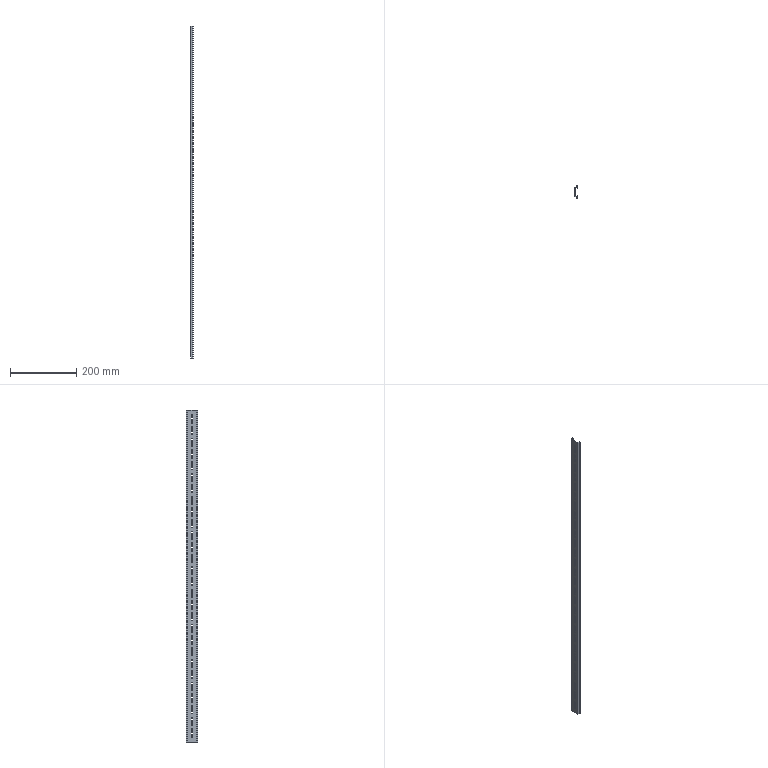Part | STEP file | SDR-1 | 1 solid | 126 faces | box 7.5 x 35 x 1000 mm | volume 65958 mm3 | plane 70 | cylinder 56 | commonest cylinder face diameters 4.5 x56